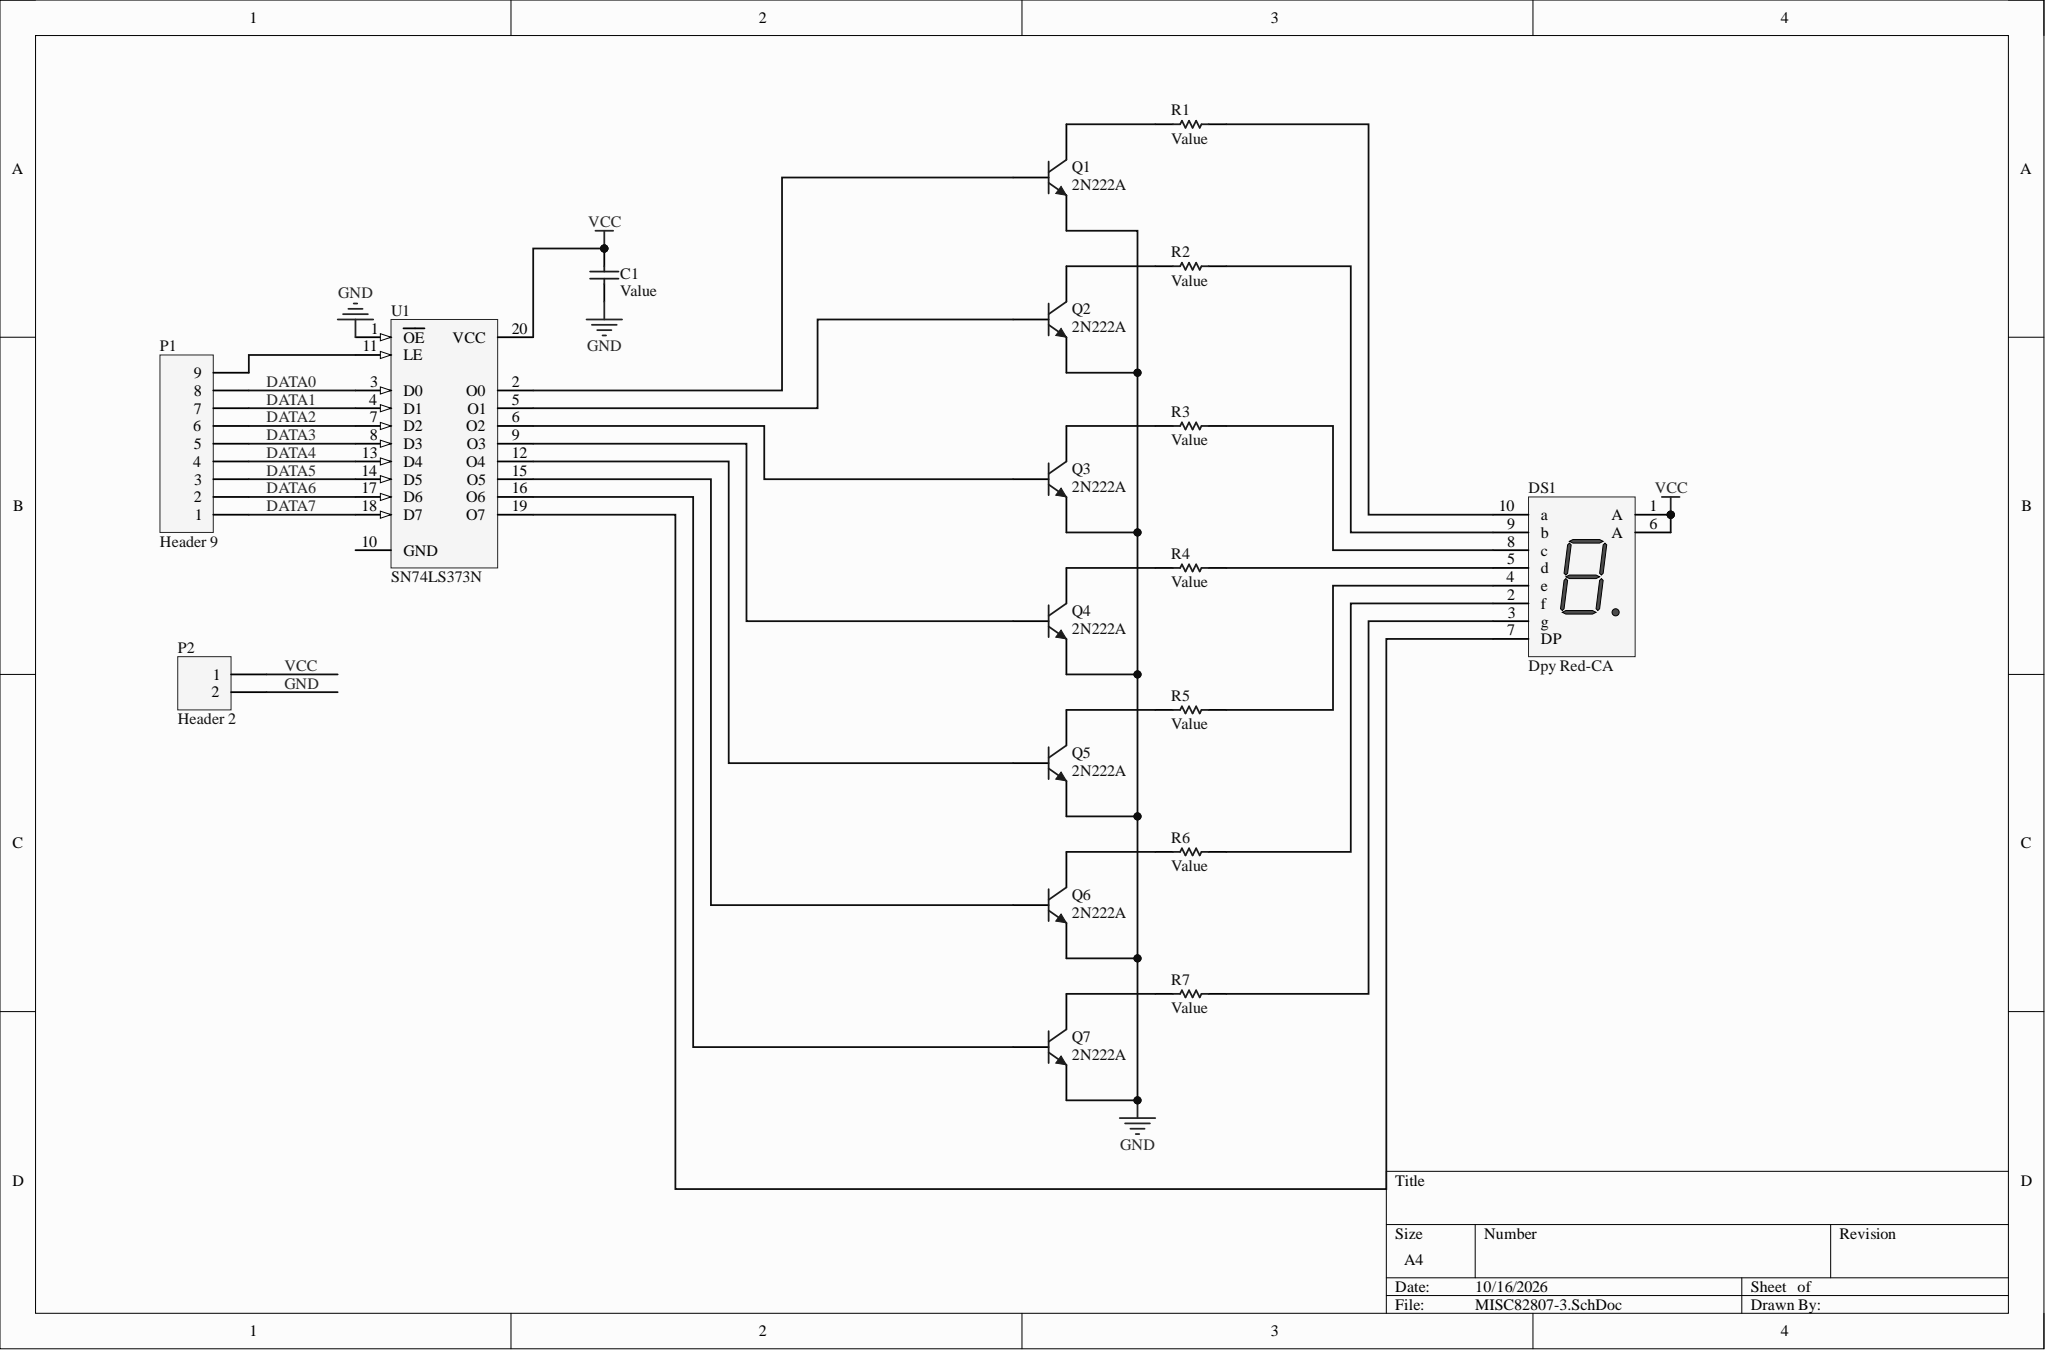Circuit board | Altium Designer | 19 parts | 33 nets
Bill of materials:
Comment,Description,Designator,Footprint,LibRef,Quantity
"Value","Capacitor","C1","RAD-0.3","Cap","1"
"Dpy Red-CA","7.62 mm Black Surface HER 7-Segment Display: CA, RH DP","DS1","A","Dpy Red-CA","1"
"Header 9","Header, 9-Pin","P1","HDR1X9","Header 9","1"
"Header 2","Header, 2-Pin","P2","HDR1X2","Header 2","1"
"2N222A","NPN General Purpose Amplifier","Q1, Q2, Q3, Q4, Q5, Q6, Q7","TO-92A","2N3904","7"
"Value","Resistor","R1, R2, R3, R4, R5, R6, R7","AXIAL-0.3","Res1","7"
"SN74LS373N","Octal Transparent Latch with 3-State Outputs","U1","738-03","SN74LS373N","1"
Netlist (Protel format):
[
C1
RAD-0.3
Value



]
[
DS1
A
Dpy Red-CA



]
[
P1
HDR1X9
Header 9



]
[
P2
HDR1X2
Header 2



]
[
Q1
TO-92A
2N222A



]
[
Q2
TO-92A
2N222A



]
[
Q3
TO-92A
2N222A



]
[
Q4
TO-92A
2N222A



]
[
Q5
TO-92A
2N222A



]
[
Q6
TO-92A
2N222A



]
[
Q7
TO-92A
2N222A



]
[
R1
AXIAL-0.3
Value



]
[
R2
AXIAL-0.3
Value



]
[
R3
AXIAL-0.3
Value



]
[
R4
AXIAL-0.3
Value



]
[
R5
AXIAL-0.3
Value



]
[
R6
AXIAL-0.3
Value



]
[
R7
AXIAL-0.3
Value



]
[
U1
738-03
SN74LS373N



]
(
VCC
C1-2
DS1-1
DS1-6
P2-1
U1-20
)
(
NetQ7_3
Q7-3
R7-1
)
(
NetQ7_2
Q7-2
U1-16
)
(
NetQ6_3
Q6-3
R6-1
)
(
NetQ6_2
Q6-2
U1-15
)
(
NetQ5_3
Q5-3
R5-1
)
(
NetQ5_2
Q5-2
U1-12
)
(
NetQ4_3
Q4-3
R4-1
)
(
NetQ4_2
Q4-2
U1-9
)
(
NetQ3_3
Q3-3
R3-1
)
(
NetQ3_2
Q3-2
U1-6
)
(
NetQ2_3
Q2-3
R2-1
)
(
NetQ2_2
Q2-2
U1-5
)
(
NetQ1_3
Q1-3
R1-1
)
(
NetQ1_2
Q1-2
U1-2
)
(
NetP1_9
P1-9
U1-11
)
(
NetDS1_10
DS1-10
R1-2
)
(
NetDS1_9
DS1-9
R2-2
)
(
NetDS1_8
DS1-8
R3-2
)
(
NetDS1_7
DS1-7
U1-19
)
(
NetDS1_5
DS1-5
R4-2
)
(
NetDS1_4
DS1-4
R5-2
)
(
NetDS1_3
DS1-3
R7-2
)
(
NetDS1_2
DS1-2
R6-2
)
(
GND
C1-1
P2-2
Q1-1
Q2-1
Q3-1
Q4-1
Q5-1
Q6-1
Q7-1
U1-1
)
(
DATA7
P1-1
U1-18
)
(
DATA6
P1-2
U1-17
)
(
DATA5
P1-3
U1-14
)
(
DATA4
P1-4
U1-13
)
(
DATA3
P1-5
U1-8
)
(
DATA2
P1-6
U1-7
)
(
DATA1
P1-7
U1-4
)
(
DATA0
P1-8
U1-3
)